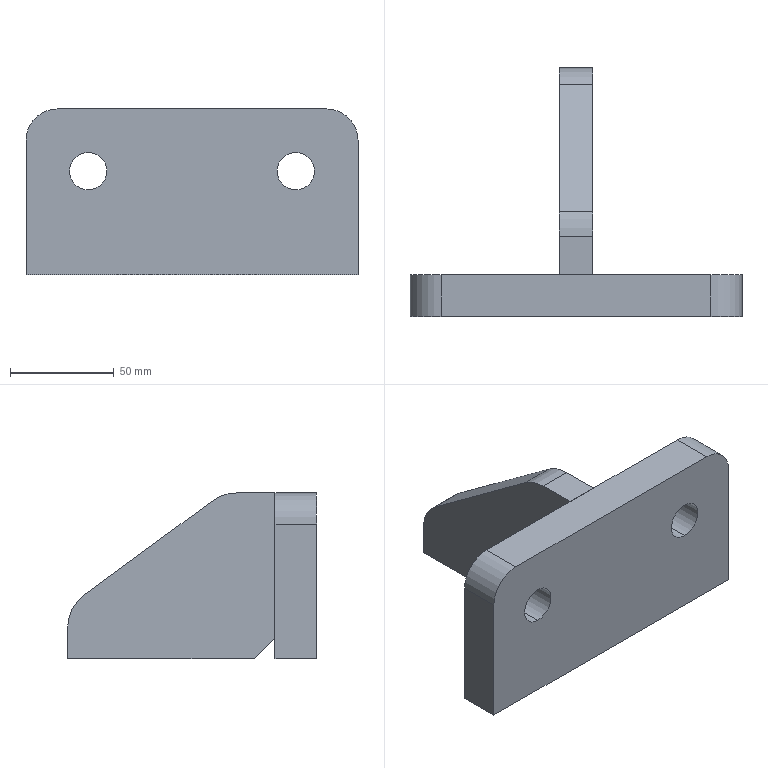Part | SolidWorks | features BaseBody 2 | 2 solids | 22 faces | box 160 x 120 x 80 mm | volume 337778 mm3 | plane 14 | cylinder 8 | commonest cylinder face diameters 18 x4 30 x2 40 x2
STEP:
#1=CARTESIAN_POINT('',(50.,10.,1.));
#2=VERTEX_POINT('',#1);
#3=CARTESIAN_POINT('',(50.,10.,19.));
#4=VERTEX_POINT('',#3);
#5=CARTESIAN_POINT('',(50.,10.,10.));
#6=DIRECTION('',(0.,1.,0.));
#7=DIRECTION('',(0.,0.,1.));
#8=AXIS2_PLACEMENT_3D('',#5,#6,#7);
#9=CIRCLE('',#8,9.);
#10=EDGE_CURVE('',#2,#4,#9,.T.);
#11=ORIENTED_EDGE('',*,*,#10,.T.);
#12=CARTESIAN_POINT('',(50.,-10.,19.));
#13=VERTEX_POINT('',#12);
#14=CARTESIAN_POINT('',(50.,10.,19.));
#15=DIRECTION('',(0.,-1.,0.));
#16=VECTOR('',#15,1000.);
#17=LINE('',#14,#16);
#18=EDGE_CURVE('',#4,#13,#17,.T.);
#19=ORIENTED_EDGE('',*,*,#18,.T.);
#20=CARTESIAN_POINT('',(50.,-10.,1.));
#21=VERTEX_POINT('',#20);
#22=CARTESIAN_POINT('',(50.,-10.,10.));
#23=DIRECTION('',(0.,1.,0.));
#24=DIRECTION('',(0.,0.,1.));
#25=AXIS2_PLACEMENT_3D('',#22,#23,#24);
#26=CIRCLE('',#25,9.);
#27=EDGE_CURVE('',#21,#13,#26,.T.);
#28=ORIENTED_EDGE('',*,*,#27,.F.);
#29=CARTESIAN_POINT('',(50.,10.,1.));
#30=DIRECTION('',(0.,-1.,0.));
#31=VECTOR('',#30,1000.);
#32=LINE('',#29,#31);
#33=EDGE_CURVE('',#2,#21,#32,.T.);
#34=ORIENTED_EDGE('',*,*,#33,.F.);
#35=EDGE_LOOP('',(#11,#19,#28,#34));
#36=FACE_OUTER_BOUND('',#35,.T.);
#37=CARTESIAN_POINT('',(50.,10.,10.));
#38=DIRECTION('',(0.,-1.,0.));
#39=DIRECTION('',(0.,0.,-1.));
#40=AXIS2_PLACEMENT_3D('',#37,#38,#39);
#41=CYLINDRICAL_SURFACE('',#40,9.);
#42=ADVANCED_FACE('',(#36),#41,.F.);
#43=CARTESIAN_POINT('',(-50.,10.,1.));
#44=VERTEX_POINT('',#43);
#45=CARTESIAN_POINT('',(-50.,10.,19.));
#46=VERTEX_POINT('',#45);
#47=CARTESIAN_POINT('',(-50.,10.,10.));
#48=DIRECTION('',(0.,1.,0.));
#49=DIRECTION('',(0.,0.,1.));
#50=AXIS2_PLACEMENT_3D('',#47,#48,#49);
#51=CIRCLE('',#50,9.);
#52=EDGE_CURVE('',#44,#46,#51,.T.);
#53=ORIENTED_EDGE('',*,*,#52,.T.);
#54=CARTESIAN_POINT('',(-50.,-10.,19.));
#55=VERTEX_POINT('',#54);
#56=CARTESIAN_POINT('',(-50.,10.,19.));
#57=DIRECTION('',(0.,-1.,0.));
#58=VECTOR('',#57,1000.);
#59=LINE('',#56,#58);
#60=EDGE_CURVE('',#46,#55,#59,.T.);
#61=ORIENTED_EDGE('',*,*,#60,.T.);
#62=CARTESIAN_POINT('',(-50.,-10.,1.));
#63=VERTEX_POINT('',#62);
#64=CARTESIAN_POINT('',(-50.,-10.,10.));
#65=DIRECTION('',(0.,1.,0.));
#66=DIRECTION('',(0.,0.,1.));
#67=AXIS2_PLACEMENT_3D('',#64,#65,#66);
#68=CIRCLE('',#67,9.);
#69=EDGE_CURVE('',#63,#55,#68,.T.);
#70=ORIENTED_EDGE('',*,*,#69,.F.);
#71=CARTESIAN_POINT('',(-50.,10.,1.));
#72=DIRECTION('',(0.,-1.,0.));
#73=VECTOR('',#72,1000.);
#74=LINE('',#71,#73);
#75=EDGE_CURVE('',#44,#63,#74,.T.);
#76=ORIENTED_EDGE('',*,*,#75,.F.);
#77=EDGE_LOOP('',(#53,#61,#70,#76));
#78=FACE_OUTER_BOUND('',#77,.T.);
#79=CARTESIAN_POINT('',(-50.,10.,10.));
#80=DIRECTION('',(0.,-1.,0.));
#81=DIRECTION('',(0.,0.,-1.));
#82=AXIS2_PLACEMENT_3D('',#79,#80,#81);
#83=CYLINDRICAL_SURFACE('',#82,9.);
#84=ADVANCED_FACE('',(#78),#83,.F.);
#85=ORIENTED_EDGE('',*,*,#52,.F.);
#86=CARTESIAN_POINT('',(-50.,10.,10.));
#87=DIRECTION('',(0.,1.,0.));
#88=DIRECTION('',(0.,0.,1.));
#89=AXIS2_PLACEMENT_3D('',#86,#87,#88);
#90=CIRCLE('',#89,9.);
#91=EDGE_CURVE('',#46,#44,#90,.T.);
#92=ORIENTED_EDGE('',*,*,#91,.F.);
#93=EDGE_LOOP('',(#85,#92));
#94=FACE_BOUND('',#93,.T.);
#95=CARTESIAN_POINT('',(-80.,10.,-40.));
#96=VERTEX_POINT('',#95);
#97=CARTESIAN_POINT('',(-80.,10.,25.));
#98=VERTEX_POINT('',#97);
#99=CARTESIAN_POINT('',(-80.,10.,-40.));
#100=DIRECTION('',(0.,0.,1.));
#101=VECTOR('',#100,1000.);
#102=LINE('',#99,#101);
#103=EDGE_CURVE('',#96,#98,#102,.T.);
#104=ORIENTED_EDGE('',*,*,#103,.T.);
#105=CARTESIAN_POINT('',(-65.,10.,40.));
#106=VERTEX_POINT('',#105);
#107=CARTESIAN_POINT('',(-65.,10.,25.));
#108=DIRECTION('',(0.,1.,0.));
#109=DIRECTION('',(0.,0.,1.));
#110=AXIS2_PLACEMENT_3D('',#107,#108,#109);
#111=CIRCLE('',#110,15.);
#112=EDGE_CURVE('',#98,#106,#111,.T.);
#113=ORIENTED_EDGE('',*,*,#112,.T.);
#114=CARTESIAN_POINT('',(65.,10.,40.));
#115=VERTEX_POINT('',#114);
#116=CARTESIAN_POINT('',(-65.,10.,40.));
#117=DIRECTION('',(1.,0.,0.));
#118=VECTOR('',#117,1000.);
#119=LINE('',#116,#118);
#120=EDGE_CURVE('',#106,#115,#119,.T.);
#121=ORIENTED_EDGE('',*,*,#120,.T.);
#122=CARTESIAN_POINT('',(80.,10.,25.));
#123=VERTEX_POINT('',#122);
#124=CARTESIAN_POINT('',(65.,10.,25.));
#125=DIRECTION('',(0.,1.,0.));
#126=DIRECTION('',(0.,0.,1.));
#127=AXIS2_PLACEMENT_3D('',#124,#125,#126);
#128=CIRCLE('',#127,15.);
#129=EDGE_CURVE('',#115,#123,#128,.T.);
#130=ORIENTED_EDGE('',*,*,#129,.T.);
#131=CARTESIAN_POINT('',(80.,10.,-40.));
#132=VERTEX_POINT('',#131);
#133=CARTESIAN_POINT('',(80.,10.,-40.));
#134=DIRECTION('',(0.,0.,-1.));
#135=VECTOR('',#134,1000.);
#136=LINE('',#133,#135);
#137=EDGE_CURVE('',#123,#132,#136,.T.);
#138=ORIENTED_EDGE('',*,*,#137,.T.);
#139=CARTESIAN_POINT('',(-80.,10.,-40.));
#140=DIRECTION('',(-1.,0.,0.));
#141=VECTOR('',#140,1000.);
#142=LINE('',#139,#141);
#143=EDGE_CURVE('',#132,#96,#142,.T.);
#144=ORIENTED_EDGE('',*,*,#143,.T.);
#145=EDGE_LOOP('',(#104,#113,#121,#130,#138,#144));
#146=FACE_OUTER_BOUND('',#145,.T.);
#147=ORIENTED_EDGE('',*,*,#10,.F.);
#148=CARTESIAN_POINT('',(50.,10.,10.));
#149=DIRECTION('',(0.,1.,0.));
#150=DIRECTION('',(0.,0.,1.));
#151=AXIS2_PLACEMENT_3D('',#148,#149,#150);
#152=CIRCLE('',#151,9.);
#153=EDGE_CURVE('',#4,#2,#152,.T.);
#154=ORIENTED_EDGE('',*,*,#153,.F.);
#155=EDGE_LOOP('',(#147,#154));
#156=FACE_BOUND('',#155,.T.);
#157=CARTESIAN_POINT('',(-65.,10.,25.));
#158=DIRECTION('',(0.,1.,0.));
#159=DIRECTION('',(0.,0.,1.));
#160=AXIS2_PLACEMENT_3D('',#157,#158,#159);
#161=PLANE('',#160);
#162=ADVANCED_FACE('',(#94,#146,#156),#161,.T.);
#163=CARTESIAN_POINT('',(-80.,-10.,-40.));
#164=VERTEX_POINT('',#163);
#165=CARTESIAN_POINT('',(-80.,-10.,25.));
#166=VERTEX_POINT('',#165);
#167=CARTESIAN_POINT('',(-80.,-10.,-40.));
#168=DIRECTION('',(0.,0.,1.));
#169=VECTOR('',#168,1000.);
#170=LINE('',#167,#169);
#171=EDGE_CURVE('',#164,#166,#170,.T.);
#172=ORIENTED_EDGE('',*,*,#171,.F.);
#173=CARTESIAN_POINT('',(80.,-10.,-40.));
#174=VERTEX_POINT('',#173);
#175=CARTESIAN_POINT('',(-80.,-10.,-40.));
#176=DIRECTION('',(-1.,0.,0.));
#177=VECTOR('',#176,1000.);
#178=LINE('',#175,#177);
#179=EDGE_CURVE('',#174,#164,#178,.T.);
#180=ORIENTED_EDGE('',*,*,#179,.F.);
#181=CARTESIAN_POINT('',(80.,-10.,25.));
#182=VERTEX_POINT('',#181);
#183=CARTESIAN_POINT('',(80.,-10.,-40.));
#184=DIRECTION('',(0.,0.,-1.));
#185=VECTOR('',#184,1000.);
#186=LINE('',#183,#185);
#187=EDGE_CURVE('',#182,#174,#186,.T.);
#188=ORIENTED_EDGE('',*,*,#187,.F.);
#189=CARTESIAN_POINT('',(65.,-10.,40.));
#190=VERTEX_POINT('',#189);
#191=CARTESIAN_POINT('',(65.,-10.,25.));
#192=DIRECTION('',(0.,1.,0.));
#193=DIRECTION('',(0.,0.,1.));
#194=AXIS2_PLACEMENT_3D('',#191,#192,#193);
#195=CIRCLE('',#194,15.);
#196=EDGE_CURVE('',#190,#182,#195,.T.);
#197=ORIENTED_EDGE('',*,*,#196,.F.);
#198=CARTESIAN_POINT('',(-65.,-10.,40.));
#199=VERTEX_POINT('',#198);
#200=CARTESIAN_POINT('',(-65.,-10.,40.));
#201=DIRECTION('',(1.,0.,0.));
#202=VECTOR('',#201,1000.);
#203=LINE('',#200,#202);
#204=EDGE_CURVE('',#199,#190,#203,.T.);
#205=ORIENTED_EDGE('',*,*,#204,.F.);
#206=CARTESIAN_POINT('',(-65.,-10.,25.));
#207=DIRECTION('',(0.,1.,0.));
#208=DIRECTION('',(0.,0.,1.));
#209=AXIS2_PLACEMENT_3D('',#206,#207,#208);
#210=CIRCLE('',#209,15.);
#211=EDGE_CURVE('',#166,#199,#210,.T.);
#212=ORIENTED_EDGE('',*,*,#211,.F.);
#213=EDGE_LOOP('',(#172,#180,#188,#197,#205,#212));
#214=FACE_OUTER_BOUND('',#213,.T.);
#215=ORIENTED_EDGE('',*,*,#69,.T.);
#216=CARTESIAN_POINT('',(-50.,-10.,10.));
#217=DIRECTION('',(0.,1.,0.));
#218=DIRECTION('',(0.,0.,1.));
#219=AXIS2_PLACEMENT_3D('',#216,#217,#218);
#220=CIRCLE('',#219,9.);
#221=EDGE_CURVE('',#55,#63,#220,.T.);
#222=ORIENTED_EDGE('',*,*,#221,.T.);
#223=EDGE_LOOP('',(#215,#222));
#224=FACE_BOUND('',#223,.T.);
#225=ORIENTED_EDGE('',*,*,#27,.T.);
#226=CARTESIAN_POINT('',(50.,-10.,10.));
#227=DIRECTION('',(0.,1.,0.));
#228=DIRECTION('',(0.,0.,1.));
#229=AXIS2_PLACEMENT_3D('',#226,#227,#228);
#230=CIRCLE('',#229,9.);
#231=EDGE_CURVE('',#13,#21,#230,.T.);
#232=ORIENTED_EDGE('',*,*,#231,.T.);
#233=EDGE_LOOP('',(#225,#232));
#234=FACE_BOUND('',#233,.T.);
#235=CARTESIAN_POINT('',(-65.,-10.,25.));
#236=DIRECTION('',(0.,1.,0.));
#237=DIRECTION('',(0.,0.,1.));
#238=AXIS2_PLACEMENT_3D('',#235,#236,#237);
#239=PLANE('',#238);
#240=ADVANCED_FACE('',(#214,#224,#234),#239,.F.);
#241=ORIENTED_EDGE('',*,*,#171,.T.);
#242=CARTESIAN_POINT('',(-80.,10.,25.));
#243=DIRECTION('',(0.,-1.,0.));
#244=VECTOR('',#243,1000.);
#245=LINE('',#242,#244);
#246=EDGE_CURVE('',#98,#166,#245,.T.);
#247=ORIENTED_EDGE('',*,*,#246,.F.);
#248=ORIENTED_EDGE('',*,*,#103,.F.);
#249=CARTESIAN_POINT('',(-80.,10.,-40.));
#250=DIRECTION('',(0.,-1.,0.));
#251=VECTOR('',#250,1000.);
#252=LINE('',#249,#251);
#253=EDGE_CURVE('',#96,#164,#252,.T.);
#254=ORIENTED_EDGE('',*,*,#253,.T.);
#255=EDGE_LOOP('',(#241,#247,#248,#254));
#256=FACE_OUTER_BOUND('',#255,.T.);
#257=CARTESIAN_POINT('',(-80.,10.,-40.));
#258=DIRECTION('',(1.,0.,0.));
#259=DIRECTION('',(0.,0.,-1.));
#260=AXIS2_PLACEMENT_3D('',#257,#258,#259);
#261=PLANE('',#260);
#262=ADVANCED_FACE('',(#256),#261,.F.);
#263=ORIENTED_EDGE('',*,*,#211,.T.);
#264=CARTESIAN_POINT('',(-65.,10.,40.));
#265=DIRECTION('',(0.,-1.,0.));
#266=VECTOR('',#265,1000.);
#267=LINE('',#264,#266);
#268=EDGE_CURVE('',#106,#199,#267,.T.);
#269=ORIENTED_EDGE('',*,*,#268,.F.);
#270=ORIENTED_EDGE('',*,*,#112,.F.);
#271=ORIENTED_EDGE('',*,*,#246,.T.);
#272=EDGE_LOOP('',(#263,#269,#270,#271));
#273=FACE_OUTER_BOUND('',#272,.T.);
#274=CARTESIAN_POINT('',(-65.,10.,25.));
#275=DIRECTION('',(0.,-1.,0.));
#276=DIRECTION('',(0.,0.,-1.));
#277=AXIS2_PLACEMENT_3D('',#274,#275,#276);
#278=CYLINDRICAL_SURFACE('',#277,15.);
#279=ADVANCED_FACE('',(#273),#278,.T.);
#280=ORIENTED_EDGE('',*,*,#204,.T.);
#281=CARTESIAN_POINT('',(65.,10.,40.));
#282=DIRECTION('',(0.,-1.,0.));
#283=VECTOR('',#282,1000.);
#284=LINE('',#281,#283);
#285=EDGE_CURVE('',#115,#190,#284,.T.);
#286=ORIENTED_EDGE('',*,*,#285,.F.);
#287=ORIENTED_EDGE('',*,*,#120,.F.);
#288=ORIENTED_EDGE('',*,*,#268,.T.);
#289=EDGE_LOOP('',(#280,#286,#287,#288));
#290=FACE_OUTER_BOUND('',#289,.T.);
#291=CARTESIAN_POINT('',(-65.,10.,40.));
#292=DIRECTION('',(0.,0.,-1.));
#293=DIRECTION('',(-1.,0.,0.));
#294=AXIS2_PLACEMENT_3D('',#291,#292,#293);
#295=PLANE('',#294);
#296=ADVANCED_FACE('',(#290),#295,.F.);
#297=ORIENTED_EDGE('',*,*,#196,.T.);
#298=CARTESIAN_POINT('',(80.,10.,25.));
#299=DIRECTION('',(0.,-1.,0.));
#300=VECTOR('',#299,1000.);
#301=LINE('',#298,#300);
#302=EDGE_CURVE('',#123,#182,#301,.T.);
#303=ORIENTED_EDGE('',*,*,#302,.F.);
#304=ORIENTED_EDGE('',*,*,#129,.F.);
#305=ORIENTED_EDGE('',*,*,#285,.T.);
#306=EDGE_LOOP('',(#297,#303,#304,#305));
#307=FACE_OUTER_BOUND('',#306,.T.);
#308=CARTESIAN_POINT('',(65.,10.,25.));
#309=DIRECTION('',(0.,-1.,0.));
#310=DIRECTION('',(0.,0.,-1.));
#311=AXIS2_PLACEMENT_3D('',#308,#309,#310);
#312=CYLINDRICAL_SURFACE('',#311,15.);
#313=ADVANCED_FACE('',(#307),#312,.T.);
#314=ORIENTED_EDGE('',*,*,#187,.T.);
#315=CARTESIAN_POINT('',(80.,10.,-40.));
#316=DIRECTION('',(0.,-1.,0.));
#317=VECTOR('',#316,1000.);
#318=LINE('',#315,#317);
#319=EDGE_CURVE('',#132,#174,#318,.T.);
#320=ORIENTED_EDGE('',*,*,#319,.F.);
#321=ORIENTED_EDGE('',*,*,#137,.F.);
#322=ORIENTED_EDGE('',*,*,#302,.T.);
#323=EDGE_LOOP('',(#314,#320,#321,#322));
#324=FACE_OUTER_BOUND('',#323,.T.);
#325=CARTESIAN_POINT('',(80.,10.,-40.));
#326=DIRECTION('',(-1.,0.,0.));
#327=DIRECTION('',(0.,0.,1.));
#328=AXIS2_PLACEMENT_3D('',#325,#326,#327);
#329=PLANE('',#328);
#330=ADVANCED_FACE('',(#324),#329,.F.);
#331=ORIENTED_EDGE('',*,*,#179,.T.);
#332=ORIENTED_EDGE('',*,*,#253,.F.);
#333=ORIENTED_EDGE('',*,*,#143,.F.);
#334=ORIENTED_EDGE('',*,*,#319,.T.);
#335=EDGE_LOOP('',(#331,#332,#333,#334));
#336=FACE_OUTER_BOUND('',#335,.T.);
#337=CARTESIAN_POINT('',(-80.,10.,-40.));
#338=DIRECTION('',(0.,0.,1.));
#339=DIRECTION('',(1.,0.,0.));
#340=AXIS2_PLACEMENT_3D('',#337,#338,#339);
#341=PLANE('',#340);
#342=ADVANCED_FACE('',(#336),#341,.F.);
#343=ORIENTED_EDGE('',*,*,#60,.F.);
#344=ORIENTED_EDGE('',*,*,#91,.T.);
#345=ORIENTED_EDGE('',*,*,#75,.T.);
#346=ORIENTED_EDGE('',*,*,#221,.F.);
#347=EDGE_LOOP('',(#343,#344,#345,#346));
#348=FACE_OUTER_BOUND('',#347,.T.);
#349=CARTESIAN_POINT('',(-50.,10.,10.));
#350=DIRECTION('',(0.,-1.,0.));
#351=DIRECTION('',(0.,0.,-1.));
#352=AXIS2_PLACEMENT_3D('',#349,#350,#351);
#353=CYLINDRICAL_SURFACE('',#352,9.);
#354=ADVANCED_FACE('',(#348),#353,.F.);
#355=ORIENTED_EDGE('',*,*,#18,.F.);
#356=ORIENTED_EDGE('',*,*,#153,.T.);
#357=ORIENTED_EDGE('',*,*,#33,.T.);
#358=ORIENTED_EDGE('',*,*,#231,.F.);
#359=EDGE_LOOP('',(#355,#356,#357,#358));
#360=FACE_OUTER_BOUND('',#359,.T.);
#361=CARTESIAN_POINT('',(50.,10.,10.));
#362=DIRECTION('',(0.,-1.,0.));
#363=DIRECTION('',(0.,0.,-1.));
#364=AXIS2_PLACEMENT_3D('',#361,#362,#363);
#365=CYLINDRICAL_SURFACE('',#364,9.);
#366=ADVANCED_FACE('',(#360),#365,.F.);
#367=CLOSED_SHELL('',(#42,#84,#162,#240,#262,#279,#296,#313,#330,#342,#354,#366));
#368=MANIFOLD_SOLID_BREP('',#367);
#369=CARTESIAN_POINT('',(-8.,10.,40.));
#370=VERTEX_POINT('',#369);
#371=CARTESIAN_POINT('',(-8.,10.,-30.));
#372=VERTEX_POINT('',#371);
#373=CARTESIAN_POINT('',(-8.,10.,40.));
#374=DIRECTION('',(0.,0.,-1.));
#375=VECTOR('',#374,1000.);
#376=LINE('',#373,#375);
#377=EDGE_CURVE('',#370,#372,#376,.T.);
#378=ORIENTED_EDGE('',*,*,#377,.T.);
#379=CARTESIAN_POINT('',(8.,10.,-30.));
#380=VERTEX_POINT('',#379);
#381=CARTESIAN_POINT('',(8.,10.,-30.));
#382=DIRECTION('',(-1.,0.,0.));
#383=VECTOR('',#382,1000.);
#384=LINE('',#381,#383);
#385=EDGE_CURVE('',#380,#372,#384,.T.);
#386=ORIENTED_EDGE('',*,*,#385,.F.);
#387=CARTESIAN_POINT('',(8.,10.,40.));
#388=VERTEX_POINT('',#387);
#389=CARTESIAN_POINT('',(8.,10.,40.));
#390=DIRECTION('',(0.,0.,-1.));
#391=VECTOR('',#390,1000.);
#392=LINE('',#389,#391);
#393=EDGE_CURVE('',#388,#380,#392,.T.);
#394=ORIENTED_EDGE('',*,*,#393,.F.);
#395=CARTESIAN_POINT('',(8.,10.,40.));
#396=DIRECTION('',(-1.,0.,0.));
#397=VECTOR('',#396,1000.);
#398=LINE('',#395,#397);
#399=EDGE_CURVE('',#388,#370,#398,.T.);
#400=ORIENTED_EDGE('',*,*,#399,.T.);
#401=EDGE_LOOP('',(#378,#386,#394,#400));
#402=FACE_OUTER_BOUND('',#401,.T.);
#403=CARTESIAN_POINT('',(8.,10.,40.));
#404=DIRECTION('',(0.,1.,0.));
#405=DIRECTION('',(0.,0.,1.));
#406=AXIS2_PLACEMENT_3D('',#403,#404,#405);
#407=PLANE('',#406);
#408=ADVANCED_FACE('',(#402),#407,.F.);
#409=CARTESIAN_POINT('',(-8.,20.,-40.));
#410=VERTEX_POINT('',#409);
#411=CARTESIAN_POINT('',(-8.,20.,-40.));
#412=DIRECTION('',(0.,0.7071,-0.7071));
#413=VECTOR('',#412,1000.);
#414=LINE('',#411,#413);
#415=EDGE_CURVE('',#372,#410,#414,.T.);
#416=ORIENTED_EDGE('',*,*,#415,.T.);
#417=CARTESIAN_POINT('',(8.,20.,-40.));
#418=VERTEX_POINT('',#417);
#419=CARTESIAN_POINT('',(8.,20.,-40.));
#420=DIRECTION('',(-1.,0.,0.));
#421=VECTOR('',#420,1000.);
#422=LINE('',#419,#421);
#423=EDGE_CURVE('',#418,#410,#422,.T.);
#424=ORIENTED_EDGE('',*,*,#423,.F.);
#425=CARTESIAN_POINT('',(8.,20.,-40.));
#426=DIRECTION('',(0.,0.7071,-0.7071));
#427=VECTOR('',#426,1000.);
#428=LINE('',#425,#427);
#429=EDGE_CURVE('',#380,#418,#428,.T.);
#430=ORIENTED_EDGE('',*,*,#429,.F.);
#431=ORIENTED_EDGE('',*,*,#385,.T.);
#432=EDGE_LOOP('',(#416,#424,#430,#431));
#433=FACE_OUTER_BOUND('',#432,.T.);
#434=CARTESIAN_POINT('',(8.,20.,-40.));
#435=DIRECTION('',(0.,0.7071,0.7071));
#436=DIRECTION('',(0.,-0.7071,0.7071));
#437=AXIS2_PLACEMENT_3D('',#434,#435,#436);
#438=PLANE('',#437);
#439=ADVANCED_FACE('',(#433),#438,.F.);
#440=CARTESIAN_POINT('',(-8.,110.,-40.));
#441=VERTEX_POINT('',#440);
#442=CARTESIAN_POINT('',(-8.,110.,-40.));
#443=DIRECTION('',(0.,1.,0.));
#444=VECTOR('',#443,1000.);
#445=LINE('',#442,#444);
#446=EDGE_CURVE('',#410,#441,#445,.T.);
#447=ORIENTED_EDGE('',*,*,#446,.T.);
#448=CARTESIAN_POINT('',(8.,110.,-40.));
#449=VERTEX_POINT('',#448);
#450=CARTESIAN_POINT('',(8.,110.,-40.));
#451=DIRECTION('',(-1.,0.,0.));
#452=VECTOR('',#451,1000.);
#453=LINE('',#450,#452);
#454=EDGE_CURVE('',#449,#441,#453,.T.);
#455=ORIENTED_EDGE('',*,*,#454,.F.);
#456=CARTESIAN_POINT('',(8.,110.,-40.));
#457=DIRECTION('',(0.,1.,0.));
#458=VECTOR('',#457,1000.);
#459=LINE('',#456,#458);
#460=EDGE_CURVE('',#418,#449,#459,.T.);
#461=ORIENTED_EDGE('',*,*,#460,.F.);
#462=ORIENTED_EDGE('',*,*,#423,.T.);
#463=EDGE_LOOP('',(#447,#455,#461,#462));
#464=FACE_OUTER_BOUND('',#463,.T.);
#465=CARTESIAN_POINT('',(8.,110.,-40.));
#466=DIRECTION('',(0.,0.,1.));
#467=DIRECTION('',(0.,-1.,0.));
#468=AXIS2_PLACEMENT_3D('',#465,#466,#467);
#469=PLANE('',#468);
#470=ADVANCED_FACE('',(#464),#469,.F.);
#471=CARTESIAN_POINT('',(-8.,110.,-25.135));
#472=VERTEX_POINT('',#471);
#473=CARTESIAN_POINT('',(-8.,110.,-25.135));
#474=DIRECTION('',(0.,0.,1.));
#475=VECTOR('',#474,1000.);
#476=LINE('',#473,#475);
#477=EDGE_CURVE('',#441,#472,#476,.T.);
#478=ORIENTED_EDGE('',*,*,#477,.T.);
#479=CARTESIAN_POINT('',(8.,110.,-25.135));
#480=VERTEX_POINT('',#479);
#481=CARTESIAN_POINT('',(8.,110.,-25.135));
#482=DIRECTION('',(-1.,0.,0.));
#483=VECTOR('',#482,1000.);
#484=LINE('',#481,#483);
#485=EDGE_CURVE('',#480,#472,#484,.T.);
#486=ORIENTED_EDGE('',*,*,#485,.F.);
#487=CARTESIAN_POINT('',(8.,110.,-25.135));
#488=DIRECTION('',(0.,0.,1.));
#489=VECTOR('',#488,1000.);
#490=LINE('',#487,#489);
#491=EDGE_CURVE('',#449,#480,#490,.T.);
#492=ORIENTED_EDGE('',*,*,#491,.F.);
#493=ORIENTED_EDGE('',*,*,#454,.T.);
#494=EDGE_LOOP('',(#478,#486,#492,#493));
#495=FACE_OUTER_BOUND('',#494,.T.);
#496=CARTESIAN_POINT('',(8.,110.,-25.135));
#497=DIRECTION('',(0.,-1.,0.));
#498=DIRECTION('',(0.,0.,-1.));
#499=AXIS2_PLACEMENT_3D('',#496,#497,#498);
#500=PLANE('',#499);
#501=ADVANCED_FACE('',(#495),#500,.F.);
#502=CARTESIAN_POINT('',(-8.,101.827,-9.007));
#503=VERTEX_POINT('',#502);
#504=CARTESIAN_POINT('',(-8.,90.,-25.135));
#505=DIRECTION('',(1.,0.,0.));
#506=DIRECTION('',(0.,0.,1.));
#507=AXIS2_PLACEMENT_3D('',#504,#505,#506);
#508=CIRCLE('',#507,20.);
#509=EDGE_CURVE('',#472,#503,#508,.T.);
#510=ORIENTED_EDGE('',*,*,#509,.T.);
#511=CARTESIAN_POINT('',(8.,101.827,-9.007));
#512=VERTEX_POINT('',#511);
#513=CARTESIAN_POINT('',(8.,101.827,-9.007));
#514=DIRECTION('',(-1.,0.,0.));
#515=VECTOR('',#514,1000.);
#516=LINE('',#513,#515);
#517=EDGE_CURVE('',#512,#503,#516,.T.);
#518=ORIENTED_EDGE('',*,*,#517,.F.);
#519=CARTESIAN_POINT('',(8.,90.,-25.135));
#520=DIRECTION('',(1.,0.,0.));
#521=DIRECTION('',(0.,0.,1.));
#522=AXIS2_PLACEMENT_3D('',#519,#520,#521);
#523=CIRCLE('',#522,20.);
#524=EDGE_CURVE('',#480,#512,#523,.T.);
#525=ORIENTED_EDGE('',*,*,#524,.F.);
#526=ORIENTED_EDGE('',*,*,#485,.T.);
#527=EDGE_LOOP('',(#510,#518,#525,#526));
#528=FACE_OUTER_BOUND('',#527,.T.);
#529=CARTESIAN_POINT('',(8.,90.,-25.135));
#530=DIRECTION('',(-1.,0.,0.));
#531=DIRECTION('',(0.,0.,1.));
#532=AXIS2_PLACEMENT_3D('',#529,#530,#531);
#533=CYLINDRICAL_SURFACE('',#532,20.);
#534=ADVANCED_FACE('',(#528),#533,.T.);
#535=CARTESIAN_POINT('',(-8.,40.28,36.128));
#536=VERTEX_POINT('',#535);
#537=CARTESIAN_POINT('',(-8.,40.28,36.128));
#538=DIRECTION('',(0.,-0.8064,0.5914));
#539=VECTOR('',#538,1000.);
#540=LINE('',#537,#539);
#541=EDGE_CURVE('',#503,#536,#540,.T.);
#542=ORIENTED_EDGE('',*,*,#541,.T.);
#543=CARTESIAN_POINT('',(8.,40.28,36.128));
#544=VERTEX_POINT('',#543);
#545=CARTESIAN_POINT('',(8.,40.28,36.128));
#546=DIRECTION('',(-1.,0.,0.));
#547=VECTOR('',#546,1000.);
#548=LINE('',#545,#547);
#549=EDGE_CURVE('',#544,#536,#548,.T.);
#550=ORIENTED_EDGE('',*,*,#549,.F.);
#551=CARTESIAN_POINT('',(8.,40.28,36.128));
#552=DIRECTION('',(0.,-0.8064,0.5914));
#553=VECTOR('',#552,1000.);
#554=LINE('',#551,#553);
#555=EDGE_CURVE('',#512,#544,#554,.T.);
#556=ORIENTED_EDGE('',*,*,#555,.F.);
#557=ORIENTED_EDGE('',*,*,#517,.T.);
#558=EDGE_LOOP('',(#542,#550,#556,#557));
#559=FACE_OUTER_BOUND('',#558,.T.);
#560=CARTESIAN_POINT('',(8.,40.28,36.128));
#561=DIRECTION('',(0.,-0.5914,-0.8064));
#562=DIRECTION('',(0.,0.8064,-0.5914));
#563=AXIS2_PLACEMENT_3D('',#560,#561,#562);
#564=PLANE('',#563);
#565=ADVANCED_FACE('',(#559),#564,.F.);
#566=CARTESIAN_POINT('',(-8.,28.453,40.));
#567=VERTEX_POINT('',#566);
#568=CARTESIAN_POINT('',(-8.,28.453,20.));
#569=DIRECTION('',(1.,0.,0.));
#570=DIRECTION('',(0.,0.,1.));
#571=AXIS2_PLACEMENT_3D('',#568,#569,#570);
#572=CIRCLE('',#571,20.);
#573=EDGE_CURVE('',#536,#567,#572,.T.);
#574=ORIENTED_EDGE('',*,*,#573,.T.);
#575=CARTESIAN_POINT('',(8.,28.453,40.));
#576=VERTEX_POINT('',#575);
#577=CARTESIAN_POINT('',(8.,28.453,40.));
#578=DIRECTION('',(-1.,0.,0.));
#579=VECTOR('',#578,1000.);
#580=LINE('',#577,#579);
#581=EDGE_CURVE('',#576,#567,#580,.T.);
#582=ORIENTED_EDGE('',*,*,#581,.F.);
#583=CARTESIAN_POINT('',(8.,28.453,20.));
#584=DIRECTION('',(1.,0.,0.));
#585=DIRECTION('',(0.,0.,1.));
#586=AXIS2_PLACEMENT_3D('',#583,#584,#585);
#587=CIRCLE('',#586,20.);
#588=EDGE_CURVE('',#544,#576,#587,.T.);
#589=ORIENTED_EDGE('',*,*,#588,.F.);
#590=ORIENTED_EDGE('',*,*,#549,.T.);
#591=EDGE_LOOP('',(#574,#582,#589,#590));
#592=FACE_OUTER_BOUND('',#591,.T.);
#593=CARTESIAN_POINT('',(8.,28.453,20.));
#594=DIRECTION('',(-1.,0.,0.));
#595=DIRECTION('',(0.,0.,1.));
#596=AXIS2_PLACEMENT_3D('',#593,#594,#595);
#597=CYLINDRICAL_SURFACE('',#596,20.);
#598=ADVANCED_FACE('',(#592),#597,.T.);
#599=CARTESIAN_POINT('',(-8.,10.,40.));
#600=DIRECTION('',(0.,-1.,0.));
#601=VECTOR('',#600,1000.);
#602=LINE('',#599,#601);
#603=EDGE_CURVE('',#567,#370,#602,.T.);
#604=ORIENTED_EDGE('',*,*,#603,.T.);
#605=ORIENTED_EDGE('',*,*,#399,.F.);
#606=CARTESIAN_POINT('',(8.,10.,40.));
#607=DIRECTION('',(0.,-1.,0.));
#608=VECTOR('',#607,1000.);
#609=LINE('',#606,#608);
#610=EDGE_CURVE('',#576,#388,#609,.T.);
#611=ORIENTED_EDGE('',*,*,#610,.F.);
#612=ORIENTED_EDGE('',*,*,#581,.T.);
#613=EDGE_LOOP('',(#604,#605,#611,#612));
#614=FACE_OUTER_BOUND('',#613,.T.);
#615=CARTESIAN_POINT('',(8.,10.,40.));
#616=DIRECTION('',(0.,0.,-1.));
#617=DIRECTION('',(-1.,0.,0.));
#618=AXIS2_PLACEMENT_3D('',#615,#616,#617);
#619=PLANE('',#618);
#620=ADVANCED_FACE('',(#614),#619,.F.);
#621=ORIENTED_EDGE('',*,*,#393,.T.);
#622=ORIENTED_EDGE('',*,*,#429,.T.);
#623=ORIENTED_EDGE('',*,*,#460,.T.);
#624=ORIENTED_EDGE('',*,*,#491,.T.);
#625=ORIENTED_EDGE('',*,*,#524,.T.);
#626=ORIENTED_EDGE('',*,*,#555,.T.);
#627=ORIENTED_EDGE('',*,*,#588,.T.);
#628=ORIENTED_EDGE('',*,*,#610,.T.);
#629=EDGE_LOOP('',(#621,#622,#623,#624,#625,#626,#627,#628));
#630=FACE_OUTER_BOUND('',#629,.T.);
#631=CARTESIAN_POINT('',(8.,90.,-25.135));
#632=DIRECTION('',(-1.,0.,0.));
#633=DIRECTION('',(0.,0.,1.));
#634=AXIS2_PLACEMENT_3D('',#631,#632,#633);
#635=PLANE('',#634);
#636=ADVANCED_FACE('',(#630),#635,.F.);
#637=ORIENTED_EDGE('',*,*,#377,.F.);
#638=ORIENTED_EDGE('',*,*,#603,.F.);
#639=ORIENTED_EDGE('',*,*,#573,.F.);
#640=ORIENTED_EDGE('',*,*,#541,.F.);
#641=ORIENTED_EDGE('',*,*,#509,.F.);
#642=ORIENTED_EDGE('',*,*,#477,.F.);
#643=ORIENTED_EDGE('',*,*,#446,.F.);
#644=ORIENTED_EDGE('',*,*,#415,.F.);
#645=EDGE_LOOP('',(#637,#638,#639,#640,#641,#642,#643,#644));
#646=FACE_OUTER_BOUND('',#645,.T.);
#647=CARTESIAN_POINT('',(-8.,90.,-25.135));
#648=DIRECTION('',(-1.,0.,0.));
#649=DIRECTION('',(0.,0.,1.));
#650=AXIS2_PLACEMENT_3D('',#647,#648,#649);
#651=PLANE('',#650);
#652=ADVANCED_FACE('',(#646),#651,.T.);
#653=CLOSED_SHELL('',(#408,#439,#470,#501,#534,#565,#598,#620,#636,#652));
#654=MANIFOLD_SOLID_BREP('',#653);
#655=CARTESIAN_POINT('',(0.,0.,0.));
#656=DIRECTION('',(0.,0.,1.));
#657=DIRECTION('',(1.,0.,0.));
#658=AXIS2_PLACEMENT_3D('',#655,#656,#657);
#659=(LENGTH_UNIT()NAMED_UNIT(*)SI_UNIT(.MILLI.,.METRE.));
#660=UNCERTAINTY_MEASURE_WITH_UNIT(LENGTH_MEASURE(0.00001),#659,'','');
#661=(NAMED_UNIT(*)PLANE_ANGLE_UNIT()SI_UNIT($,.RADIAN.));
#662=(NAMED_UNIT(*)SI_UNIT($,.STERADIAN.)SOLID_ANGLE_UNIT());
#663=(GEOMETRIC_REPRESENTATION_CONTEXT(3)GLOBAL_UNCERTAINTY_ASSIGNED_CONTEXT((#660))GLOBAL_UNIT_ASSIGNED_CONTEXT((#659,#661,#662))REPRESENTATION_CONTEXT('',''));
#664=ADVANCED_BREP_SHAPE_REPRESENTATION('',(#368,#654,#658),#663);